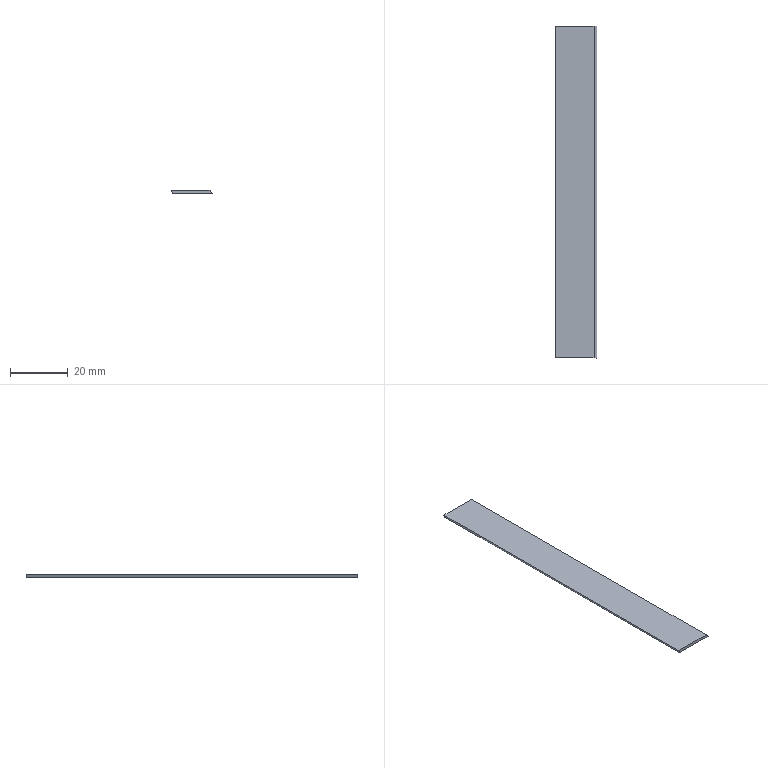Part | SolidWorks | features BaseBody 1 | 1 solid | 6 faces | box 14.371 x 115.104 x 1.056 mm | volume 1662 mm3 | plane 4 | cylinder 2 | commonest cylinder face diameters 97.2 x1 165.792 x1
STEP:
#1=CARTESIAN_POINT('',(-2168.709,1269.344,-1610.536));
#2=VERTEX_POINT('',#1);
#3=CARTESIAN_POINT('',(-2168.709,1154.24,-1610.536));
#4=VERTEX_POINT('',#3);
#5=CARTESIAN_POINT('',(-2168.709,1269.344,-1610.536));
#6=DIRECTION('',(0.,-1.,0.));
#7=VECTOR('',#6,1000.);
#8=LINE('',#5,#7);
#9=EDGE_CURVE('',#2,#4,#8,.T.);
#10=ORIENTED_EDGE('',*,*,#9,.F.);
#11=CARTESIAN_POINT('',(-2169.653,1269.344,-1609.48));
#12=VERTEX_POINT('',#11);
#13=CARTESIAN_POINT('',(-2132.95,1269.344,-1577.624));
#14=DIRECTION('',(0.,1.,0.));
#15=DIRECTION('',(-0.7358,0.,-0.6772));
#16=AXIS2_PLACEMENT_3D('',#13,#14,#15);
#17=CIRCLE('',#16,48.6);
#18=EDGE_CURVE('',#2,#12,#17,.T.);
#19=ORIENTED_EDGE('',*,*,#18,.T.);
#20=CARTESIAN_POINT('',(-2169.653,1154.24,-1609.48));
#21=VERTEX_POINT('',#20);
#22=CARTESIAN_POINT('',(-2169.653,1269.344,-1609.48));
#23=DIRECTION('',(0.,-1.,0.));
#24=VECTOR('',#23,1000.);
#25=LINE('',#22,#24);
#26=EDGE_CURVE('',#12,#21,#25,.T.);
#27=ORIENTED_EDGE('',*,*,#26,.T.);
#28=CARTESIAN_POINT('',(-2132.95,1154.24,-1577.624));
#29=DIRECTION('',(0.,-1.,0.));
#30=DIRECTION('',(-0.7552,0.,-0.6555));
#31=AXIS2_PLACEMENT_3D('',#28,#29,#30);
#32=CIRCLE('',#31,48.6);
#33=EDGE_CURVE('',#21,#4,#32,.T.);
#34=ORIENTED_EDGE('',*,*,#33,.T.);
#35=EDGE_LOOP('',(#10,#19,#27,#34));
#36=FACE_OUTER_BOUND('',#35,.T.);
#37=CARTESIAN_POINT('',(-2132.95,1275.099,-1577.624));
#38=DIRECTION('',(0.,-1.,0.));
#39=DIRECTION('',(-0.8095,0.,-0.5872));
#40=AXIS2_PLACEMENT_3D('',#37,#38,#39);
#41=CYLINDRICAL_SURFACE('',#40,48.6);
#42=ADVANCED_FACE('',(#36),#41,.F.);
#43=CARTESIAN_POINT('',(-2182.632,1269.344,-1610.536));
#44=VERTEX_POINT('',#43);
#45=CARTESIAN_POINT('',(-2182.632,1154.24,-1610.536));
#46=VERTEX_POINT('',#45);
#47=CARTESIAN_POINT('',(-2182.632,1269.344,-1610.536));
#48=DIRECTION('',(0.,-1.,0.));
#49=VECTOR('',#48,1000.);
#50=LINE('',#47,#49);
#51=EDGE_CURVE('',#44,#46,#50,.T.);
#52=ORIENTED_EDGE('',*,*,#51,.T.);
#53=CARTESIAN_POINT('',(-2183.08,1154.24,-1609.48));
#54=VERTEX_POINT('',#53);
#55=CARTESIAN_POINT('',(-2106.55,1154.24,-1577.624));
#56=DIRECTION('',(0.,-1.,0.));
#57=DIRECTION('',(-0.9232,0.,-0.3843));
#58=AXIS2_PLACEMENT_3D('',#55,#56,#57);
#59=CIRCLE('',#58,82.896);
#60=EDGE_CURVE('',#54,#46,#59,.T.);
#61=ORIENTED_EDGE('',*,*,#60,.F.);
#62=CARTESIAN_POINT('',(-2183.08,1269.344,-1609.48));
#63=VERTEX_POINT('',#62);
#64=CARTESIAN_POINT('',(-2183.08,1154.24,-1609.48));
#65=DIRECTION('',(0.,1.,0.));
#66=VECTOR('',#65,1000.);
#67=LINE('',#64,#66);
#68=EDGE_CURVE('',#54,#63,#67,.T.);
#69=ORIENTED_EDGE('',*,*,#68,.T.);
#70=CARTESIAN_POINT('',(-2106.55,1269.344,-1577.624));
#71=DIRECTION('',(0.,1.,0.));
#72=DIRECTION('',(-0.9178,0.,-0.397));
#73=AXIS2_PLACEMENT_3D('',#70,#71,#72);
#74=CIRCLE('',#73,82.896);
#75=EDGE_CURVE('',#44,#63,#74,.T.);
#76=ORIENTED_EDGE('',*,*,#75,.F.);
#77=EDGE_LOOP('',(#52,#61,#69,#76));
#78=FACE_OUTER_BOUND('',#77,.T.);
#79=CARTESIAN_POINT('',(-2106.55,1275.099,-1577.624));
#80=DIRECTION('',(0.,1.,0.));
#81=DIRECTION('',(-0.8797,0.,-0.4755));
#82=AXIS2_PLACEMENT_3D('',#79,#80,#81);
#83=CYLINDRICAL_SURFACE('',#82,82.896);
#84=ADVANCED_FACE('',(#78),#83,.T.);
#85=ORIENTED_EDGE('',*,*,#9,.T.);
#86=CARTESIAN_POINT('',(-2182.632,1154.24,-1610.536));
#87=DIRECTION('',(1.,0.,-0.000000012));
#88=VECTOR('',#87,1000.);
#89=LINE('',#86,#88);
#90=EDGE_CURVE('',#46,#4,#89,.T.);
#91=ORIENTED_EDGE('',*,*,#90,.F.);
#92=ORIENTED_EDGE('',*,*,#51,.F.);
#93=CARTESIAN_POINT('',(-2168.709,1269.344,-1610.536));
#94=DIRECTION('',(-1.,0.,0.000000012));
#95=VECTOR('',#94,1000.);
#96=LINE('',#93,#95);
#97=EDGE_CURVE('',#2,#44,#96,.T.);
#98=ORIENTED_EDGE('',*,*,#97,.F.);
#99=EDGE_LOOP('',(#85,#91,#92,#98));
#100=FACE_OUTER_BOUND('',#99,.T.);
#101=CARTESIAN_POINT('',(-2188.387,1275.099,-1610.536));
#102=DIRECTION('',(0.,0.,-1.));
#103=DIRECTION('',(0.,-1.,0.));
#104=AXIS2_PLACEMENT_3D('',#101,#102,#103);
#105=PLANE('',#104);
#106=ADVANCED_FACE('',(#100),#105,.T.);
#107=ORIENTED_EDGE('',*,*,#18,.F.);
#108=ORIENTED_EDGE('',*,*,#97,.T.);
#109=ORIENTED_EDGE('',*,*,#75,.T.);
#110=CARTESIAN_POINT('',(-2183.08,1269.344,-1609.48));
#111=DIRECTION('',(1.,0.000000002,0.000000003));
#112=VECTOR('',#111,1000.);
#113=LINE('',#110,#112);
#114=EDGE_CURVE('',#63,#12,#113,.T.);
#115=ORIENTED_EDGE('',*,*,#114,.T.);
#116=EDGE_LOOP('',(#107,#108,#109,#115));
#117=FACE_OUTER_BOUND('',#116,.T.);
#118=CARTESIAN_POINT('',(-2183.799,1269.344,-1611.255));
#119=DIRECTION('',(0.,1.,0.));
#120=DIRECTION('',(1.,0.,0.));
#121=AXIS2_PLACEMENT_3D('',#118,#119,#120);
#122=PLANE('',#121);
#123=ADVANCED_FACE('',(#117),#122,.T.);
#124=ORIENTED_EDGE('',*,*,#68,.F.);
#125=CARTESIAN_POINT('',(-2169.653,1154.24,-1609.48));
#126=DIRECTION('',(-1.,0.,-0.000000007));
#127=VECTOR('',#126,1000.);
#128=LINE('',#125,#127);
#129=EDGE_CURVE('',#21,#54,#128,.T.);
#130=ORIENTED_EDGE('',*,*,#129,.F.);
#131=ORIENTED_EDGE('',*,*,#26,.F.);
#132=ORIENTED_EDGE('',*,*,#114,.F.);
#133=EDGE_LOOP('',(#124,#130,#131,#132));
#134=FACE_OUTER_BOUND('',#133,.T.);
#135=CARTESIAN_POINT('',(-2163.898,1275.099,-1609.48));
#136=DIRECTION('',(0.,0.,1.));
#137=DIRECTION('',(1.,0.,0.));
#138=AXIS2_PLACEMENT_3D('',#135,#136,#137);
#139=PLANE('',#138);
#140=ADVANCED_FACE('',(#134),#139,.T.);
#141=ORIENTED_EDGE('',*,*,#33,.F.);
#142=ORIENTED_EDGE('',*,*,#129,.T.);
#143=ORIENTED_EDGE('',*,*,#60,.T.);
#144=ORIENTED_EDGE('',*,*,#90,.T.);
#145=EDGE_LOOP('',(#141,#142,#143,#144));
#146=FACE_OUTER_BOUND('',#145,.T.);
#147=CARTESIAN_POINT('',(-2167.991,1154.24,-1608.762));
#148=DIRECTION('',(0.,-1.,0.));
#149=DIRECTION('',(0.,0.,-1.));
#150=AXIS2_PLACEMENT_3D('',#147,#148,#149);
#151=PLANE('',#150);
#152=ADVANCED_FACE('',(#146),#151,.T.);
#153=CLOSED_SHELL('',(#42,#84,#106,#123,#140,#152));
#154=MANIFOLD_SOLID_BREP('',#153);
#155=CARTESIAN_POINT('',(0.,0.,0.));
#156=DIRECTION('',(0.,0.,1.));
#157=DIRECTION('',(1.,0.,0.));
#158=AXIS2_PLACEMENT_3D('',#155,#156,#157);
#159=(LENGTH_UNIT()NAMED_UNIT(*)SI_UNIT(.MILLI.,.METRE.));
#160=UNCERTAINTY_MEASURE_WITH_UNIT(LENGTH_MEASURE(0.00001),#159,'','');
#161=(NAMED_UNIT(*)PLANE_ANGLE_UNIT()SI_UNIT($,.RADIAN.));
#162=(NAMED_UNIT(*)SI_UNIT($,.STERADIAN.)SOLID_ANGLE_UNIT());
#163=(GEOMETRIC_REPRESENTATION_CONTEXT(3)GLOBAL_UNCERTAINTY_ASSIGNED_CONTEXT((#160))GLOBAL_UNIT_ASSIGNED_CONTEXT((#159,#161,#162))REPRESENTATION_CONTEXT('',''));
#164=ADVANCED_BREP_SHAPE_REPRESENTATION('',(#154,#158),#163);